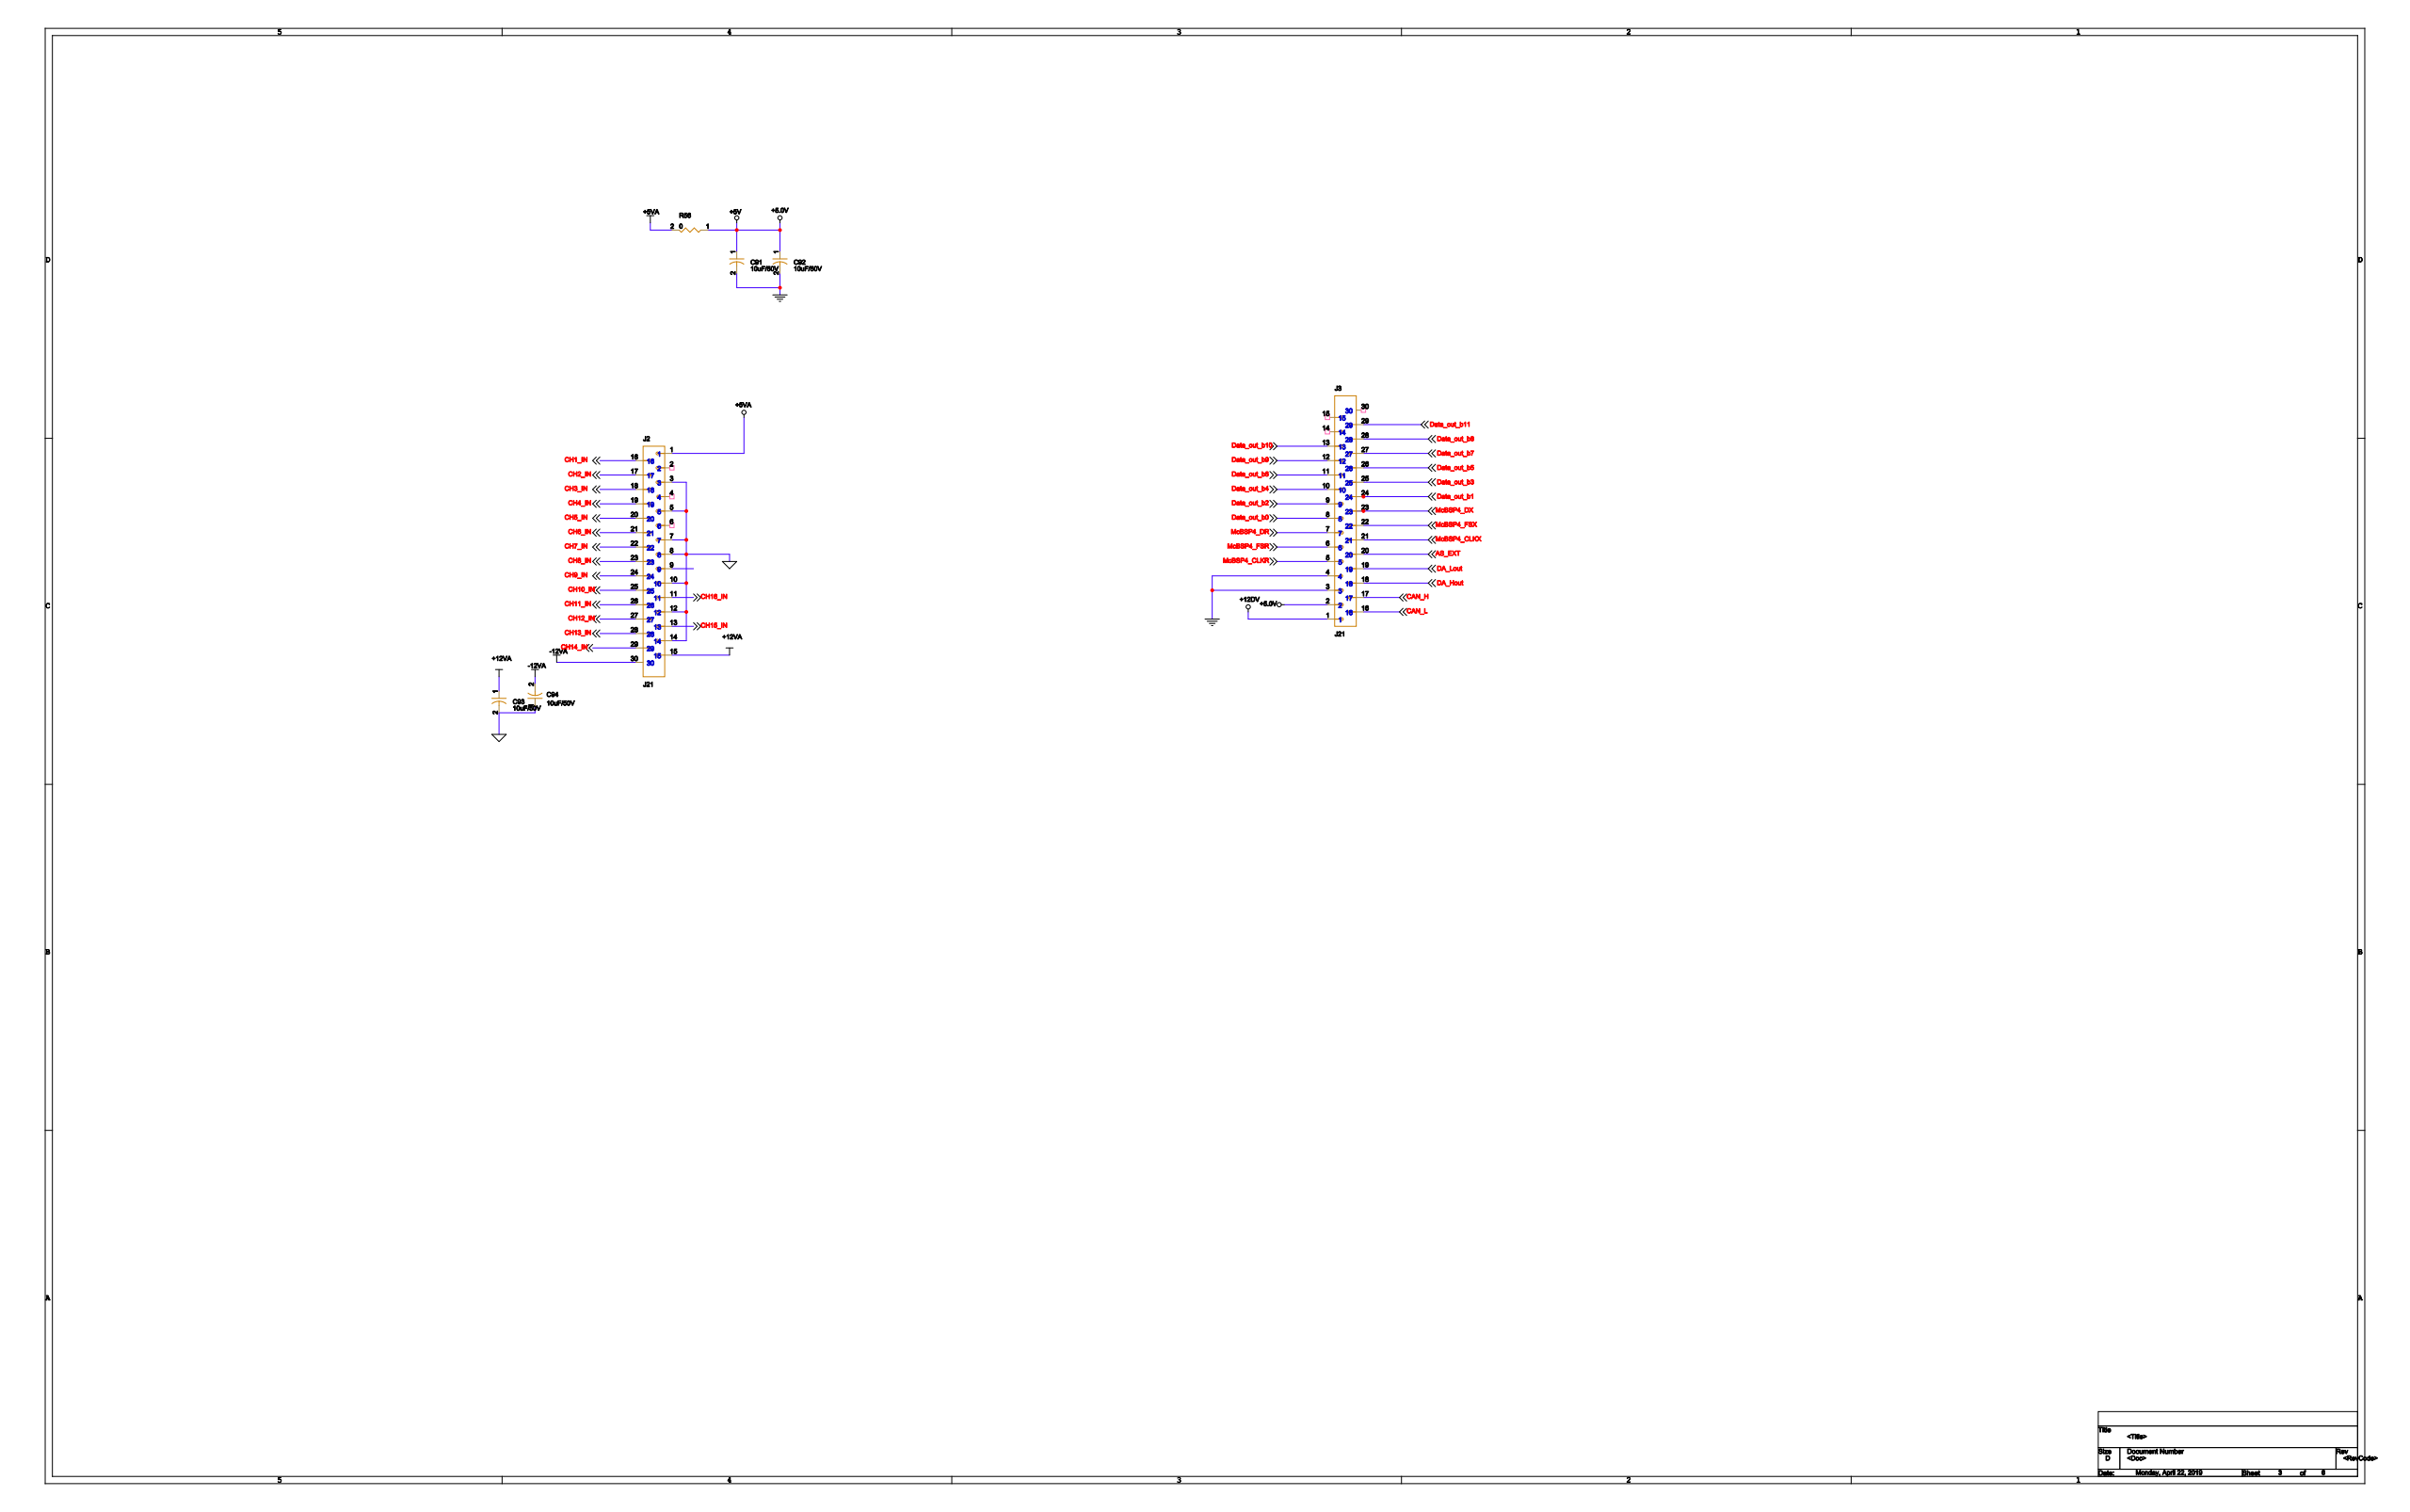Circuit board | Cadence Allegro | 362 parts | 391 nets | one sheet of the schematic
Parts on this sheet (reference | value | footprint):
C91 | 10uF/50V | 7343
C92 | 10uF/50V | 7343
C93 | 10uF/50V | 7343
C94 | 10uF/50V | 7343
J2 | J21 | GH_30M
J3 | J21 | GH_30M
R56 | 0 | 0805
Nets of these parts (net: part-pin ...):
+12VA: C93-1 J2-15
-12VA: C94-2 J2-30
DGND: C91-2 C92-2 J3-3 J3-4
AGND: C93-2 C94-1 J2-3 J2-5 J2-7 J2-8 J2-10 J2-12 J2-14
+5.0V: C91-1 C92-1 R56-1 J3-2
+5VA: R56-2 J2-1
AS_EXT: J3-20
CAN_L: J3-16
CAN_H: J3-17
+12DV: J3-1
CH16_IN: J2-11
CH15_IN: J2-13
CH1_IN: J2-16
CH2_IN: J2-17
CH3_IN: J2-18
CH4_IN: J2-19
CH5_IN: J2-20
CH6_IN: J2-21
CH7_IN: J2-22
CH8_IN: J2-23
CH9_IN: J2-24
CH10_IN: J2-25
CH11_IN: J2-26
CH12_IN: J2-27
CH13_IN: J2-28
CH14_IN: J2-29